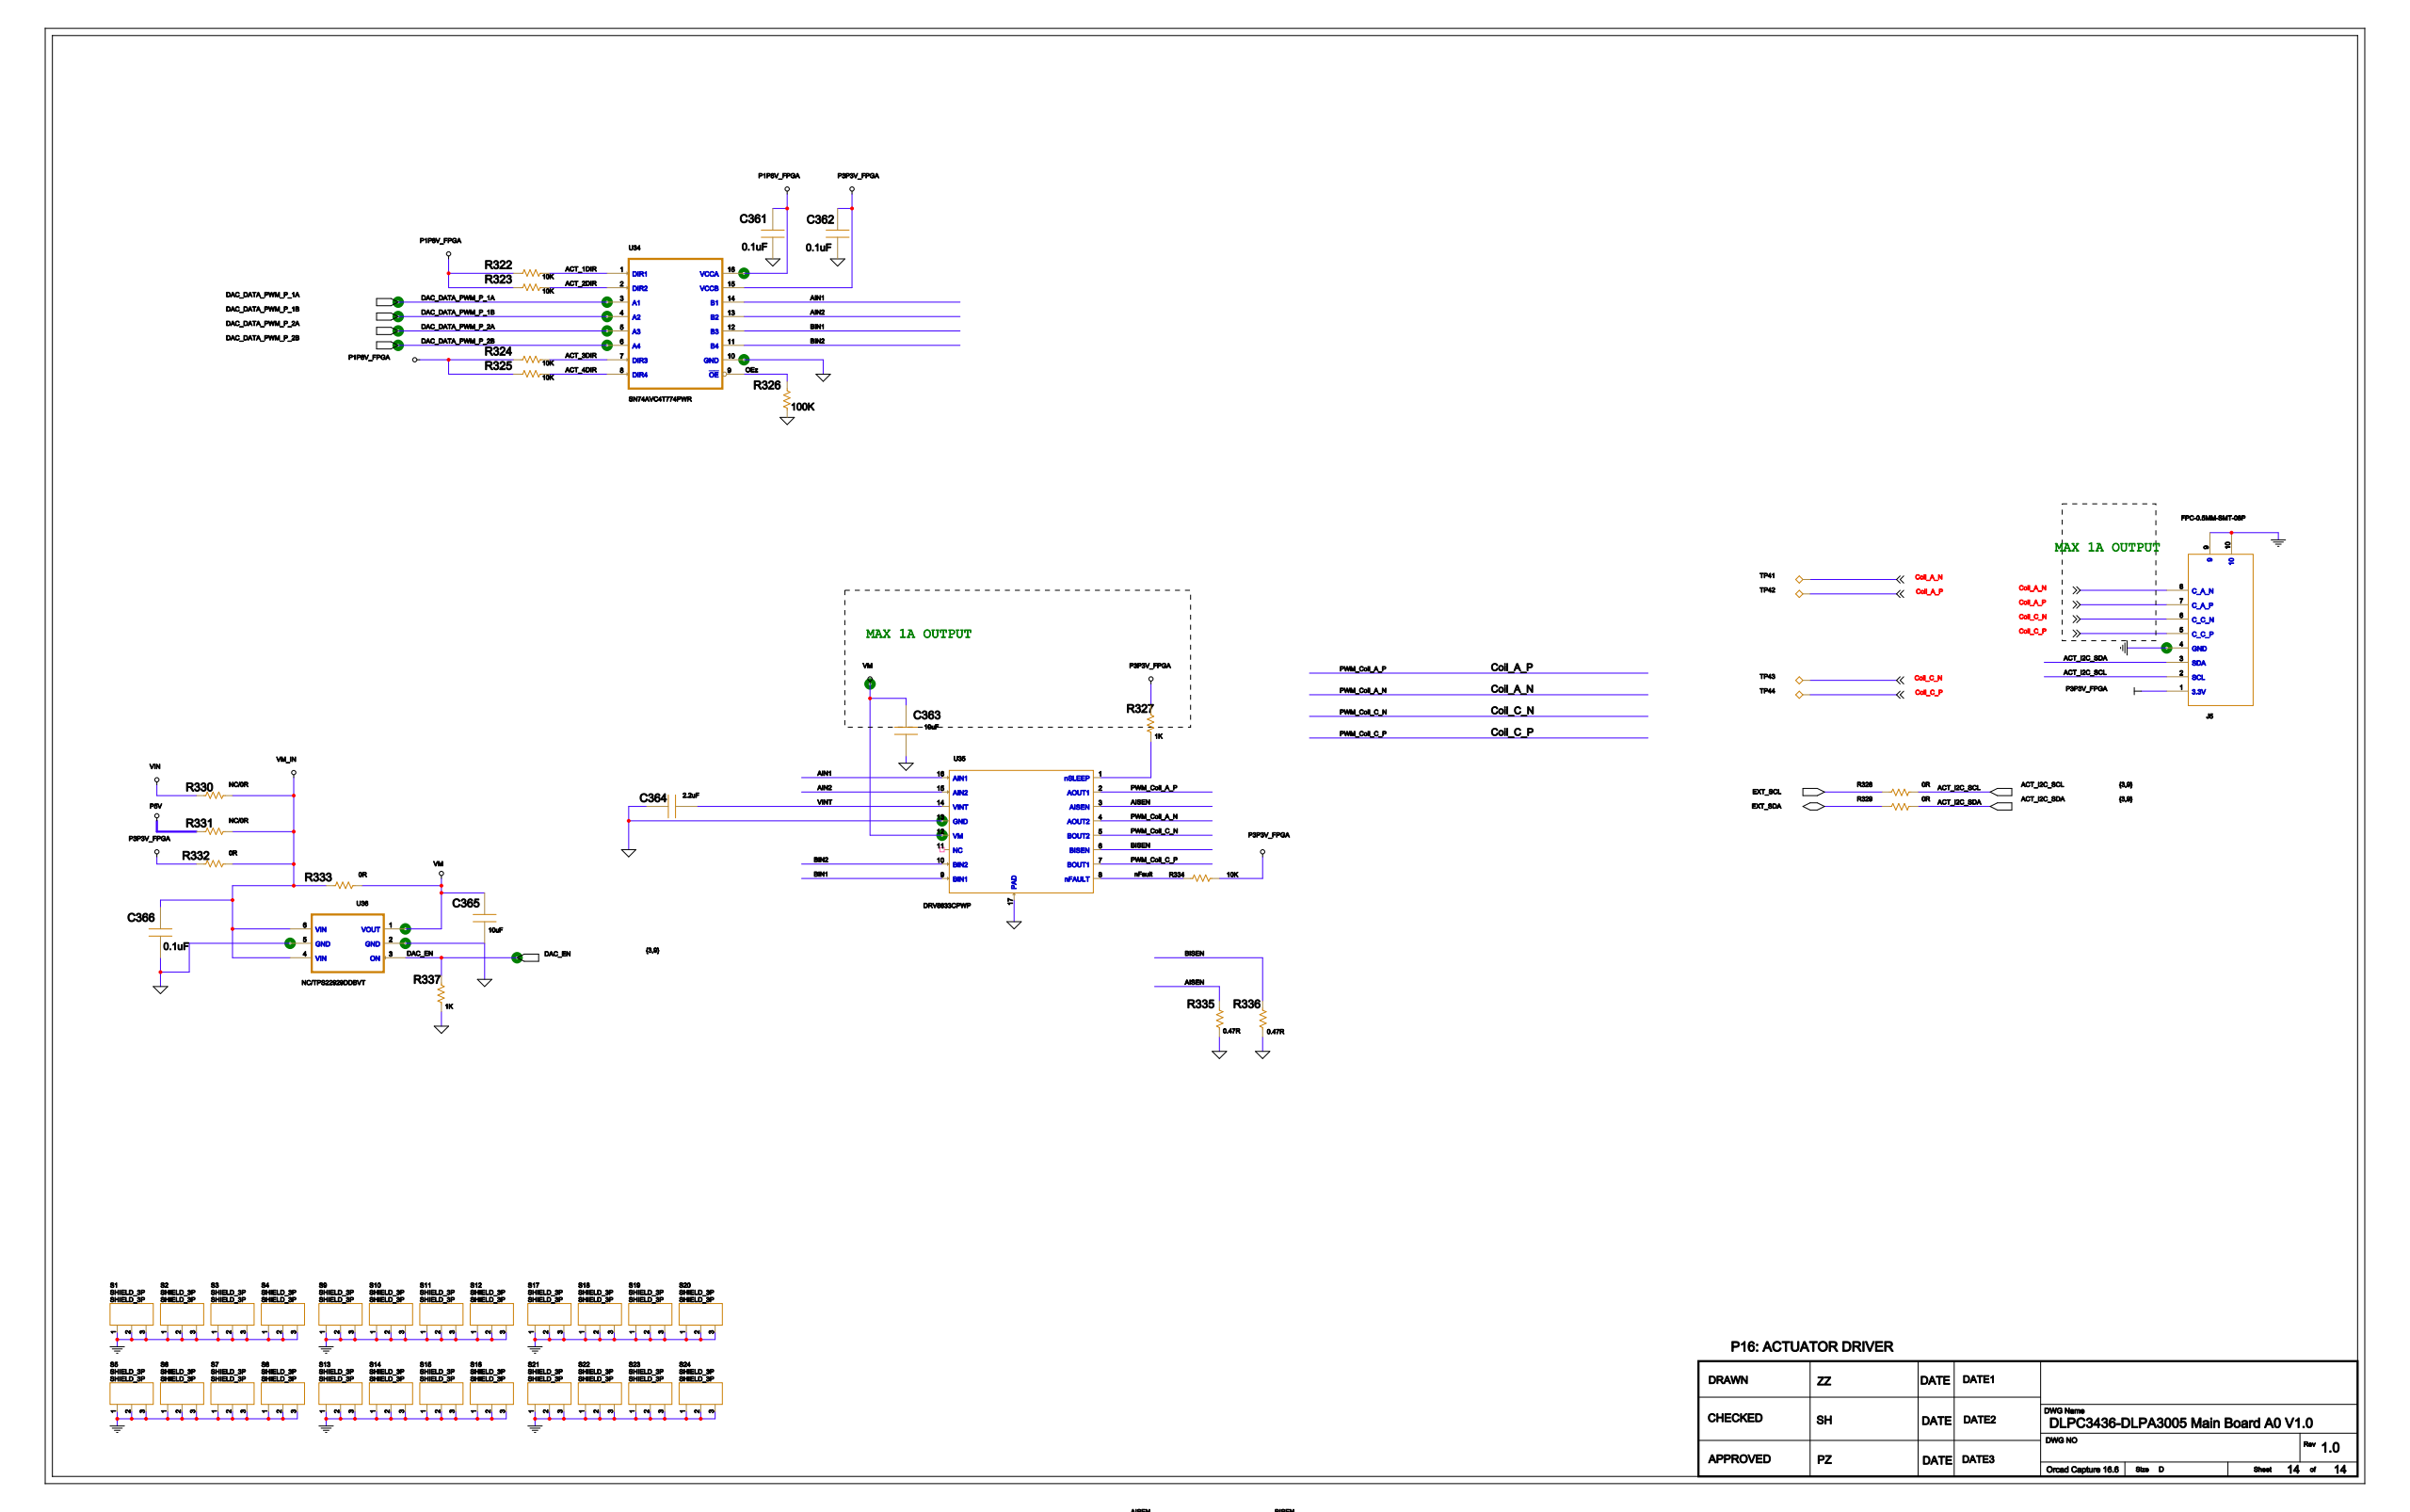Circuit board | Cadence Allegro | 1223 parts | 777 nets | one sheet of the schematic
Parts on this sheet (reference | value | footprint):
C361 | 0.1uF | C0201
C362 | 0.1uF | C0201
C363 | 10uF | C0603
C364 | 2.2uF | C0402
C365 | 10uF | C0603
C366 | 0.1uF | C0201
J5 | FPC-0.5MM-SMT-08P | 50208_0_8MM_8P
R322 | 10K | R0201
R323 | 10K | R0201
R324 | 10K | R0201
R325 | 10K | R0201
R326 | 100K | R0201
R327 | 1K | R0201
R328 | 0R | R0201
R329 | 0R | R0201
R330 | NC/0R | R0603
R331 | NC/0R | R0603
R332 | 0R | R0603
R333 | 0R | R0402
R334 | 10K | R0201
R335 | 0.47R | R0603
R336 | 0.47R | R0603
R337 | 1K | R0201
S1 | SHIELD_3P | SHIELD_3P
S2 | SHIELD_3P | SHIELD_3P
S3 | SHIELD_3P | SHIELD_3P
S4 | SHIELD_3P | SHIELD_3P
S5 | SHIELD_3P | SHIELD_3P
S6 | SHIELD_3P | SHIELD_3P
S7 | SHIELD_3P | SHIELD_3P
S8 | SHIELD_3P | SHIELD_3P
S9 | SHIELD_3P | SHIELD_3P
S10 | SHIELD_3P | SHIELD_3P
S11 | SHIELD_3P | SHIELD_3P
S12 | SHIELD_3P | SHIELD_3P
S13 | SHIELD_3P | SHIELD_3P
S14 | SHIELD_3P | SHIELD_3P
S15 | SHIELD_3P | SHIELD_3P
S16 | SHIELD_3P | SHIELD_3P
S17 | SHIELD_3P | SHIELD_3P
S18 | SHIELD_3P | SHIELD_3P
S19 | SHIELD_3P | SHIELD_3P
S20 | SHIELD_3P | SHIELD_3P
S21 | SHIELD_3P | SHIELD_3P
S22 | SHIELD_3P | SHIELD_3P
S23 | SHIELD_3P | SHIELD_3P
S24 | SHIELD_3P | SHIELD_3P
TP41 | TP40 | TP06MM
TP42 | TP40 | TP06MM
TP43 | TP40 | TP06MM
TP44 | TP40 | TP06MM
U34 | SN74AVC4T774PWR | TSSOP16_PW
U35 | DRV8833CPWP | TSSOP16-EP
U36 | NC/TPS22929DDBVT | SOT-23-6
Nets of these parts (net: part-pin ...):
GND: C361-1 C362-1 C363-2 C364-1 C365-2 C366-1 J5-4 J5-9 J5-10 R326-1 R335-2 R336-2 R337-1 S1-1 S1-2 S1-3 S2-1 S2-2 S2-3 S3-1 S3-2 S3-3 S4-1 S4-2 S4-3 S5-1 S5-2 S5-3 S6-1 S6-2 S6-3 S7-1 S7-2 S7-3 S8-1 S8-2 S8-3 S9-1 S9-2 S9-3 S10-1 S10-2 S10-3 S11-1 S11-2 S11-3 S12-1 S12-2 S12-3 S13-1 S13-2 S13-3 S14-1 S14-2 S14-3 S15-1 S15-2 S15-3 S16-1 S16-2 S16-3 S17-1 S17-2 S17-3 S18-1 S18-2 S18-3 S19-1 S19-2 S19-3 S20-1 S20-2 S20-3 S21-1 S21-2 S21-3 S22-1 S22-2 S22-3 S23-1 S23-2 S23-3 S24-1 S24-2 S24-3 U34-10 U35-13 U35-17 U36-2 U36-5
P3P3V_FPGA: C362-2 J5-1 R327-2 R332-1 R334-2 U34-15
P1P8V_FPGA: C361-2 R322-1 R323-1 R324-1 R325-1 U34-16
VM_IN: C366-2 R330-2 R331-2 R332-2 R333-1 U36-4 U36-6
VDLP: R330-1
P5V: R331-1
VM: C363-1 C365-1 R333-2 U35-12 U36-1
VINT: C364-2 U35-14
COIL_A_N: J5-8 TP41-1 U35-4
COIL_A_P: J5-7 TP42-1 U35-2
COIL_C_N: J5-6 TP43-1 U35-5
COIL_C_P: J5-5 TP44-1 U35-7
ACT_I2C_SCL: J5-2 R328-1
ACT_I2C_SDA: J5-3 R329-1
OEZ: R326-2 U34-9
EXT_SCL: R328-2
EXT_SDA: R329-2
ACT_1DIR: R322-2 U34-1
ACT_2DIR: R323-2 U34-2
ACT_3DIR: R324-2 U34-7
ACT_4DIR: R325-2 U34-8
NFAULT: R334-1 U35-8
N23786988: R327-1 U35-1
DAC_EN: R337-2 U36-3
AISEN: R335-1 U35-3
BISEN: R336-1 U35-6
DAC_DATA_PWM_P_2A: U34-5
DAC_DATA_PWM_P_1B: U34-4
DAC_DATA_PWM_P_1A: U34-3
DAC_DATA_PWM_P_2B: U34-6
AIN1: U34-14 U35-16
AIN2: U34-13 U35-15
BIN1: U34-12 U35-9
BIN2: U34-11 U35-10